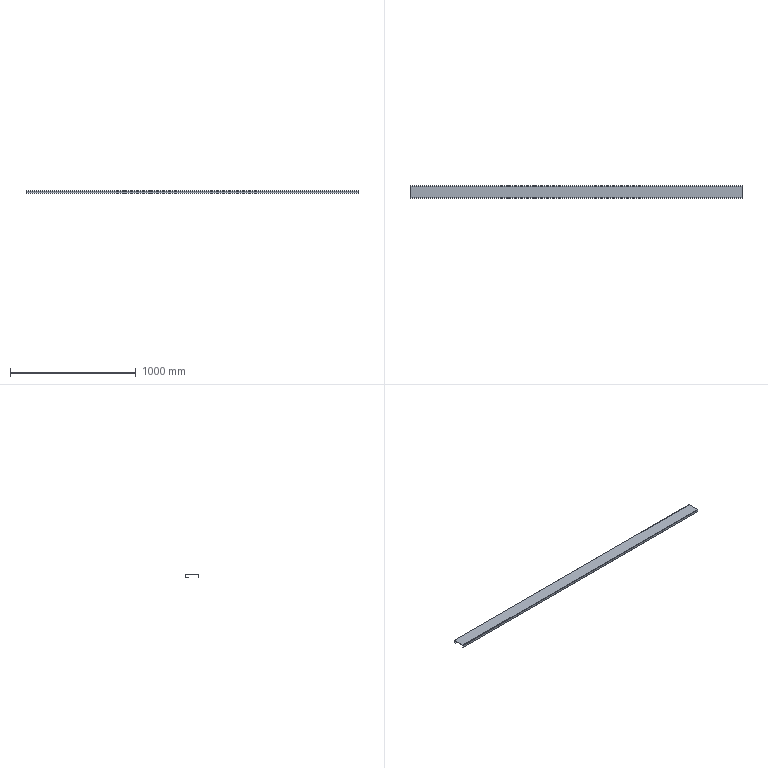Part | STEP file | E3-中转釜护栏2踢脚Plate | 1 solid | 18 faces | box 2640 x 100 x 20 mm | volume 606857 mm3 | plane 12 | cylinder 6 | commonest cylinder face diameters 2 x3 5 x3
STEP:
#1=CARTESIAN_POINT('',(0.,0.,0.));
#2=DIRECTION('',(0.,0.,1.));
#3=DIRECTION('',(1.,0.,0.));
#4=AXIS2_PLACEMENT_3D('',#1,#2,#3);
#5=CARTESIAN_POINT('',(-1320.,1.5,-2.5));
#6=VERTEX_POINT('',#5);
#7=CARTESIAN_POINT('',(-1320.,1.5,-20.));
#8=VERTEX_POINT('',#7);
#9=CARTESIAN_POINT('',(-1320.,1.5,-2.5));
#10=DIRECTION('',(0.,0.,-1.));
#11=VECTOR('',#10,1.);
#12=LINE('',#9,#11);
#13=CARTESIAN_POINT('',(1320.,1.5,-2.5));
#14=DIRECTION('',(0.,-1.,0.));
#15=DIRECTION('',(0.,0.,1.));
#16=AXIS2_PLACEMENT_3D('',#13,#14,#15);
#17=PLANE('',#16);
#18=CARTESIAN_POINT('',(0.,2640.));
#19=DIRECTION('',(-1.,0.));
#20=VECTOR('',#19,1.);
#21=LINE('',#18,#20);
#22=(GEOMETRIC_REPRESENTATION_CONTEXT(2)PARAMETRIC_REPRESENTATION_CONTEXT()REPRESENTATION_CONTEXT('',''));
#23=DEFINITIONAL_REPRESENTATION('',(#21),#22);
#24=PCURVE('',#17,#23);
#25=CARTESIAN_POINT('',(-1320.,2.5,-2.5));
#26=DIRECTION('',(-1.,0.,0.));
#27=DIRECTION('',(0.,0.,-1.));
#28=AXIS2_PLACEMENT_3D('',#25,#26,#27);
#29=PLANE('',#28);
#30=CARTESIAN_POINT('',(0.,1.));
#31=DIRECTION('',(1.,0.));
#32=VECTOR('',#31,1.);
#33=LINE('',#30,#32);
#34=(GEOMETRIC_REPRESENTATION_CONTEXT(2)PARAMETRIC_REPRESENTATION_CONTEXT()REPRESENTATION_CONTEXT('',''));
#35=DEFINITIONAL_REPRESENTATION('',(#33),#34);
#36=PCURVE('',#29,#35);
#37=SURFACE_CURVE('',#12,(#24,#36),.PCURVE_S1.);
#38=EDGE_CURVE('',#6,#8,#37,.T.);
#39=ORIENTED_EDGE('',*,*,#38,.F.);
#40=CARTESIAN_POINT('',(1320.,1.5,-2.5));
#41=VERTEX_POINT('',#40);
#42=CARTESIAN_POINT('',(1320.,1.5,-2.5));
#43=DIRECTION('',(-1.,0.,0.));
#44=VECTOR('',#43,1.);
#45=LINE('',#42,#44);
#46=CARTESIAN_POINT('',(0.,0.));
#47=DIRECTION('',(0.,1.));
#48=VECTOR('',#47,1.);
#49=LINE('',#46,#48);
#50=(GEOMETRIC_REPRESENTATION_CONTEXT(2)PARAMETRIC_REPRESENTATION_CONTEXT()REPRESENTATION_CONTEXT('',''));
#51=DEFINITIONAL_REPRESENTATION('',(#49),#50);
#52=PCURVE('',#17,#51);
#53=CARTESIAN_POINT('',(1320.,2.5,-2.5));
#54=DIRECTION('',(-1.,0.,0.));
#55=DIRECTION('',(0.,0.,-1.));
#56=AXIS2_PLACEMENT_3D('',#53,#54,#55);
#57=CYLINDRICAL_SURFACE('',#56,1.);
#58=CARTESIAN_POINT('',(1.571,0.));
#59=DIRECTION('',(0.,1.));
#60=VECTOR('',#59,1.);
#61=LINE('',#58,#60);
#62=(GEOMETRIC_REPRESENTATION_CONTEXT(2)PARAMETRIC_REPRESENTATION_CONTEXT()REPRESENTATION_CONTEXT('',''));
#63=DEFINITIONAL_REPRESENTATION('',(#61),#62);
#64=PCURVE('',#57,#63);
#65=SURFACE_CURVE('',#45,(#52,#64),.PCURVE_S1.);
#66=EDGE_CURVE('',#41,#6,#65,.T.);
#67=ORIENTED_EDGE('',*,*,#66,.F.);
#68=CARTESIAN_POINT('',(1320.,1.5,-20.));
#69=VERTEX_POINT('',#68);
#70=CARTESIAN_POINT('',(1320.,1.5,-2.5));
#71=DIRECTION('',(0.,0.,-1.));
#72=VECTOR('',#71,1.);
#73=LINE('',#70,#72);
#74=CARTESIAN_POINT('',(0.,0.));
#75=DIRECTION('',(-1.,0.));
#76=VECTOR('',#75,1.);
#77=LINE('',#74,#76);
#78=(GEOMETRIC_REPRESENTATION_CONTEXT(2)PARAMETRIC_REPRESENTATION_CONTEXT()REPRESENTATION_CONTEXT('',''));
#79=DEFINITIONAL_REPRESENTATION('',(#77),#78);
#80=PCURVE('',#17,#79);
#81=CARTESIAN_POINT('',(1320.,2.5,-2.5));
#82=DIRECTION('',(-1.,0.,0.));
#83=DIRECTION('',(0.,0.,-1.));
#84=AXIS2_PLACEMENT_3D('',#81,#82,#83);
#85=PLANE('',#84);
#86=CARTESIAN_POINT('',(0.,1.));
#87=DIRECTION('',(1.,0.));
#88=VECTOR('',#87,1.);
#89=LINE('',#86,#88);
#90=(GEOMETRIC_REPRESENTATION_CONTEXT(2)PARAMETRIC_REPRESENTATION_CONTEXT()REPRESENTATION_CONTEXT('',''));
#91=DEFINITIONAL_REPRESENTATION('',(#89),#90);
#92=PCURVE('',#85,#91);
#93=SURFACE_CURVE('',#73,(#80,#92),.PCURVE_S1.);
#94=EDGE_CURVE('',#41,#69,#93,.T.);
#95=ORIENTED_EDGE('',*,*,#94,.T.);
#96=CARTESIAN_POINT('',(1320.,1.5,-20.));
#97=DIRECTION('',(-1.,0.,0.));
#98=VECTOR('',#97,1.);
#99=LINE('',#96,#98);
#100=CARTESIAN_POINT('',(-17.5,0.));
#101=DIRECTION('',(0.,1.));
#102=VECTOR('',#101,1.);
#103=LINE('',#100,#102);
#104=(GEOMETRIC_REPRESENTATION_CONTEXT(2)PARAMETRIC_REPRESENTATION_CONTEXT()REPRESENTATION_CONTEXT('',''));
#105=DEFINITIONAL_REPRESENTATION('',(#103),#104);
#106=PCURVE('',#17,#105);
#107=CARTESIAN_POINT('',(1320.,0.,-20.));
#108=DIRECTION('',(0.,0.,-1.));
#109=DIRECTION('',(1.,0.,0.));
#110=AXIS2_PLACEMENT_3D('',#107,#108,#109);
#111=PLANE('',#110);
#112=CARTESIAN_POINT('',(0.,-1.5));
#113=DIRECTION('',(-1.,0.));
#114=VECTOR('',#113,1.);
#115=LINE('',#112,#114);
#116=(GEOMETRIC_REPRESENTATION_CONTEXT(2)PARAMETRIC_REPRESENTATION_CONTEXT()REPRESENTATION_CONTEXT('',''));
#117=DEFINITIONAL_REPRESENTATION('',(#115),#116);
#118=PCURVE('',#111,#117);
#119=SURFACE_CURVE('',#99,(#106,#118),.PCURVE_S1.);
#120=EDGE_CURVE('',#69,#8,#119,.T.);
#121=ORIENTED_EDGE('',*,*,#120,.T.);
#122=EDGE_LOOP('',(#39,#67,#95,#121));
#123=FACE_BOUND('',#122,.T.);
#124=ADVANCED_FACE('',(#123),#17,.F.);
#125=CARTESIAN_POINT('',(-1320.,0.,-20.));
#126=VERTEX_POINT('',#125);
#127=CARTESIAN_POINT('',(-1320.,0.,-20.));
#128=DIRECTION('',(0.,1.,0.));
#129=VECTOR('',#128,1.);
#130=LINE('',#127,#129);
#131=CARTESIAN_POINT('',(-2640.,0.));
#132=DIRECTION('',(0.,-1.));
#133=VECTOR('',#132,1.);
#134=LINE('',#131,#133);
#135=(GEOMETRIC_REPRESENTATION_CONTEXT(2)PARAMETRIC_REPRESENTATION_CONTEXT()REPRESENTATION_CONTEXT('',''));
#136=DEFINITIONAL_REPRESENTATION('',(#134),#135);
#137=PCURVE('',#111,#136);
#138=CARTESIAN_POINT('',(17.5,2.5));
#139=DIRECTION('',(0.,-1.));
#140=VECTOR('',#139,1.);
#141=LINE('',#138,#140);
#142=(GEOMETRIC_REPRESENTATION_CONTEXT(2)PARAMETRIC_REPRESENTATION_CONTEXT()REPRESENTATION_CONTEXT('',''));
#143=DEFINITIONAL_REPRESENTATION('',(#141),#142);
#144=PCURVE('',#29,#143);
#145=SURFACE_CURVE('',#130,(#137,#144),.PCURVE_S1.);
#146=EDGE_CURVE('',#126,#8,#145,.T.);
#147=ORIENTED_EDGE('',*,*,#146,.T.);
#148=ORIENTED_EDGE('',*,*,#120,.F.);
#149=CARTESIAN_POINT('',(1320.,0.,-20.));
#150=VERTEX_POINT('',#149);
#151=CARTESIAN_POINT('',(1320.,0.,-20.));
#152=DIRECTION('',(0.,1.,0.));
#153=VECTOR('',#152,1.);
#154=LINE('',#151,#153);
#155=CARTESIAN_POINT('',(0.,0.));
#156=DIRECTION('',(0.,-1.));
#157=VECTOR('',#156,1.);
#158=LINE('',#155,#157);
#159=(GEOMETRIC_REPRESENTATION_CONTEXT(2)PARAMETRIC_REPRESENTATION_CONTEXT()REPRESENTATION_CONTEXT('',''));
#160=DEFINITIONAL_REPRESENTATION('',(#158),#159);
#161=PCURVE('',#111,#160);
#162=CARTESIAN_POINT('',(17.5,2.5));
#163=DIRECTION('',(0.,-1.));
#164=VECTOR('',#163,1.);
#165=LINE('',#162,#164);
#166=(GEOMETRIC_REPRESENTATION_CONTEXT(2)PARAMETRIC_REPRESENTATION_CONTEXT()REPRESENTATION_CONTEXT('',''));
#167=DEFINITIONAL_REPRESENTATION('',(#165),#166);
#168=PCURVE('',#85,#167);
#169=SURFACE_CURVE('',#154,(#161,#168),.PCURVE_S1.);
#170=EDGE_CURVE('',#150,#69,#169,.T.);
#171=ORIENTED_EDGE('',*,*,#170,.F.);
#172=CARTESIAN_POINT('',(1320.,0.,-20.));
#173=DIRECTION('',(-1.,0.,0.));
#174=VECTOR('',#173,1.);
#175=LINE('',#172,#174);
#176=CARTESIAN_POINT('',(0.,0.));
#177=DIRECTION('',(-1.,0.));
#178=VECTOR('',#177,1.);
#179=LINE('',#176,#178);
#180=(GEOMETRIC_REPRESENTATION_CONTEXT(2)PARAMETRIC_REPRESENTATION_CONTEXT()REPRESENTATION_CONTEXT('',''));
#181=DEFINITIONAL_REPRESENTATION('',(#179),#180);
#182=PCURVE('',#111,#181);
#183=CARTESIAN_POINT('',(1320.,0.,-2.5));
#184=DIRECTION('',(0.,-1.,0.));
#185=DIRECTION('',(0.,0.,1.));
#186=AXIS2_PLACEMENT_3D('',#183,#184,#185);
#187=PLANE('',#186);
#188=CARTESIAN_POINT('',(-17.5,0.));
#189=DIRECTION('',(0.,1.));
#190=VECTOR('',#189,1.);
#191=LINE('',#188,#190);
#192=(GEOMETRIC_REPRESENTATION_CONTEXT(2)PARAMETRIC_REPRESENTATION_CONTEXT()REPRESENTATION_CONTEXT('',''));
#193=DEFINITIONAL_REPRESENTATION('',(#191),#192);
#194=PCURVE('',#187,#193);
#195=SURFACE_CURVE('',#175,(#182,#194),.PCURVE_S1.);
#196=EDGE_CURVE('',#150,#126,#195,.T.);
#197=ORIENTED_EDGE('',*,*,#196,.T.);
#198=EDGE_LOOP('',(#147,#148,#171,#197));
#199=FACE_BOUND('',#198,.T.);
#200=ADVANCED_FACE('',(#199),#111,.T.);
#201=CARTESIAN_POINT('',(-1320.,0.,-2.5));
#202=VERTEX_POINT('',#201);
#203=CARTESIAN_POINT('',(-1320.,0.,-2.5));
#204=DIRECTION('',(0.,0.,-1.));
#205=VECTOR('',#204,1.);
#206=LINE('',#203,#205);
#207=CARTESIAN_POINT('',(0.,2640.));
#208=DIRECTION('',(-1.,0.));
#209=VECTOR('',#208,1.);
#210=LINE('',#207,#209);
#211=(GEOMETRIC_REPRESENTATION_CONTEXT(2)PARAMETRIC_REPRESENTATION_CONTEXT()REPRESENTATION_CONTEXT('',''));
#212=DEFINITIONAL_REPRESENTATION('',(#210),#211);
#213=PCURVE('',#187,#212);
#214=CARTESIAN_POINT('',(0.,2.5));
#215=DIRECTION('',(1.,0.));
#216=VECTOR('',#215,1.);
#217=LINE('',#214,#216);
#218=(GEOMETRIC_REPRESENTATION_CONTEXT(2)PARAMETRIC_REPRESENTATION_CONTEXT()REPRESENTATION_CONTEXT('',''));
#219=DEFINITIONAL_REPRESENTATION('',(#217),#218);
#220=PCURVE('',#29,#219);
#221=SURFACE_CURVE('',#206,(#213,#220),.PCURVE_S1.);
#222=EDGE_CURVE('',#202,#126,#221,.T.);
#223=ORIENTED_EDGE('',*,*,#222,.T.);
#224=ORIENTED_EDGE('',*,*,#196,.F.);
#225=CARTESIAN_POINT('',(1320.,0.,-2.5));
#226=VERTEX_POINT('',#225);
#227=CARTESIAN_POINT('',(1320.,0.,-2.5));
#228=DIRECTION('',(0.,0.,-1.));
#229=VECTOR('',#228,1.);
#230=LINE('',#227,#229);
#231=CARTESIAN_POINT('',(0.,0.));
#232=DIRECTION('',(-1.,0.));
#233=VECTOR('',#232,1.);
#234=LINE('',#231,#233);
#235=(GEOMETRIC_REPRESENTATION_CONTEXT(2)PARAMETRIC_REPRESENTATION_CONTEXT()REPRESENTATION_CONTEXT('',''));
#236=DEFINITIONAL_REPRESENTATION('',(#234),#235);
#237=PCURVE('',#187,#236);
#238=CARTESIAN_POINT('',(0.,2.5));
#239=DIRECTION('',(1.,0.));
#240=VECTOR('',#239,1.);
#241=LINE('',#238,#240);
#242=(GEOMETRIC_REPRESENTATION_CONTEXT(2)PARAMETRIC_REPRESENTATION_CONTEXT()REPRESENTATION_CONTEXT('',''));
#243=DEFINITIONAL_REPRESENTATION('',(#241),#242);
#244=PCURVE('',#85,#243);
#245=SURFACE_CURVE('',#230,(#237,#244),.PCURVE_S1.);
#246=EDGE_CURVE('',#226,#150,#245,.T.);
#247=ORIENTED_EDGE('',*,*,#246,.F.);
#248=CARTESIAN_POINT('',(1320.,0.,-2.5));
#249=DIRECTION('',(-1.,0.,0.));
#250=VECTOR('',#249,1.);
#251=LINE('',#248,#250);
#252=CARTESIAN_POINT('',(0.,0.));
#253=DIRECTION('',(0.,1.));
#254=VECTOR('',#253,1.);
#255=LINE('',#252,#254);
#256=(GEOMETRIC_REPRESENTATION_CONTEXT(2)PARAMETRIC_REPRESENTATION_CONTEXT()REPRESENTATION_CONTEXT('',''));
#257=DEFINITIONAL_REPRESENTATION('',(#255),#256);
#258=PCURVE('',#187,#257);
#259=CARTESIAN_POINT('',(1320.,2.5,-2.5));
#260=DIRECTION('',(-1.,0.,0.));
#261=DIRECTION('',(0.,0.,-1.));
#262=AXIS2_PLACEMENT_3D('',#259,#260,#261);
#263=CYLINDRICAL_SURFACE('',#262,2.5);
#264=CARTESIAN_POINT('',(1.571,0.));
#265=DIRECTION('',(0.,1.));
#266=VECTOR('',#265,1.);
#267=LINE('',#264,#266);
#268=(GEOMETRIC_REPRESENTATION_CONTEXT(2)PARAMETRIC_REPRESENTATION_CONTEXT()REPRESENTATION_CONTEXT('',''));
#269=DEFINITIONAL_REPRESENTATION('',(#267),#268);
#270=PCURVE('',#263,#269);
#271=SURFACE_CURVE('',#251,(#258,#270),.PCURVE_S1.);
#272=EDGE_CURVE('',#226,#202,#271,.T.);
#273=ORIENTED_EDGE('',*,*,#272,.T.);
#274=EDGE_LOOP('',(#223,#224,#247,#273));
#275=FACE_BOUND('',#274,.T.);
#276=ADVANCED_FACE('',(#275),#187,.T.);
#277=CARTESIAN_POINT('',(-1320.,2.5,0.));
#278=VERTEX_POINT('',#277);
#279=CARTESIAN_POINT('',(-1320.,2.5,-2.5));
#280=DIRECTION('',(1.,0.,0.));
#281=DIRECTION('',(0.,0.,-1.));
#282=AXIS2_PLACEMENT_3D('',#279,#280,#281);
#283=CIRCLE('',#282,2.5);
#284=CARTESIAN_POINT('',(6.283,2640.));
#285=DIRECTION('',(-1.,0.));
#286=VECTOR('',#285,1.);
#287=LINE('',#284,#286);
#288=(GEOMETRIC_REPRESENTATION_CONTEXT(2)PARAMETRIC_REPRESENTATION_CONTEXT()REPRESENTATION_CONTEXT('',''));
#289=DEFINITIONAL_REPRESENTATION('',(#287),#288);
#290=PCURVE('',#263,#289);
#291=CARTESIAN_POINT('',(2.5,0.));
#292=CARTESIAN_POINT('',(2.5,-4.33));
#293=CARTESIAN_POINT('',(-1.25,-2.165));
#294=CARTESIAN_POINT('',(-5.,0.));
#295=CARTESIAN_POINT('',(-1.25,2.165));
#296=CARTESIAN_POINT('',(2.5,4.33));
#297=CARTESIAN_POINT('',(2.5,0.));
#298=(BOUNDED_CURVE()B_SPLINE_CURVE(2,(#291,#292,#293,#294,#295,#296,#297),.UNSPECIFIED.,.T.,.F.)B_SPLINE_CURVE_WITH_KNOTS((1,2,2,2,2,1),(-2.094,0.,2.094,4.189,6.283,8.378),.UNSPECIFIED.)CURVE()GEOMETRIC_REPRESENTATION_ITEM()RATIONAL_B_SPLINE_CURVE((1.,0.5,1.,0.5,1.,0.5,1.))REPRESENTATION_ITEM(''));
#299=(GEOMETRIC_REPRESENTATION_CONTEXT(2)PARAMETRIC_REPRESENTATION_CONTEXT()REPRESENTATION_CONTEXT('',''));
#300=DEFINITIONAL_REPRESENTATION('',(#298),#299);
#301=PCURVE('',#29,#300);
#302=SURFACE_CURVE('',#283,(#290,#301),.PCURVE_S1.);
#303=EDGE_CURVE('',#278,#202,#302,.T.);
#304=ORIENTED_EDGE('',*,*,#303,.T.);
#305=ORIENTED_EDGE('',*,*,#272,.F.);
#306=CARTESIAN_POINT('',(1320.,2.5,0.));
#307=VERTEX_POINT('',#306);
#308=CARTESIAN_POINT('',(1320.,2.5,-2.5));
#309=DIRECTION('',(1.,0.,0.));
#310=DIRECTION('',(0.,0.,-1.));
#311=AXIS2_PLACEMENT_3D('',#308,#309,#310);
#312=CIRCLE('',#311,2.5);
#313=CARTESIAN_POINT('',(6.283,0.));
#314=DIRECTION('',(-1.,0.));
#315=VECTOR('',#314,1.);
#316=LINE('',#313,#315);
#317=(GEOMETRIC_REPRESENTATION_CONTEXT(2)PARAMETRIC_REPRESENTATION_CONTEXT()REPRESENTATION_CONTEXT('',''));
#318=DEFINITIONAL_REPRESENTATION('',(#316),#317);
#319=PCURVE('',#263,#318);
#320=CARTESIAN_POINT('',(2.5,0.));
#321=CARTESIAN_POINT('',(2.5,-4.33));
#322=CARTESIAN_POINT('',(-1.25,-2.165));
#323=CARTESIAN_POINT('',(-5.,0.));
#324=CARTESIAN_POINT('',(-1.25,2.165));
#325=CARTESIAN_POINT('',(2.5,4.33));
#326=CARTESIAN_POINT('',(2.5,0.));
#327=(BOUNDED_CURVE()B_SPLINE_CURVE(2,(#320,#321,#322,#323,#324,#325,#326),.UNSPECIFIED.,.T.,.F.)B_SPLINE_CURVE_WITH_KNOTS((1,2,2,2,2,1),(-2.094,0.,2.094,4.189,6.283,8.378),.UNSPECIFIED.)CURVE()GEOMETRIC_REPRESENTATION_ITEM()RATIONAL_B_SPLINE_CURVE((1.,0.5,1.,0.5,1.,0.5,1.))REPRESENTATION_ITEM(''));
#328=(GEOMETRIC_REPRESENTATION_CONTEXT(2)PARAMETRIC_REPRESENTATION_CONTEXT()REPRESENTATION_CONTEXT('',''));
#329=DEFINITIONAL_REPRESENTATION('',(#327),#328);
#330=PCURVE('',#85,#329);
#331=SURFACE_CURVE('',#312,(#319,#330),.PCURVE_S1.);
#332=EDGE_CURVE('',#307,#226,#331,.T.);
#333=ORIENTED_EDGE('',*,*,#332,.F.);
#334=CARTESIAN_POINT('',(1320.,2.5,0.));
#335=DIRECTION('',(-1.,0.,0.));
#336=VECTOR('',#335,1.);
#337=LINE('',#334,#336);
#338=CARTESIAN_POINT('',(3.142,0.));
#339=DIRECTION('',(0.,1.));
#340=VECTOR('',#339,1.);
#341=LINE('',#338,#340);
#342=(GEOMETRIC_REPRESENTATION_CONTEXT(2)PARAMETRIC_REPRESENTATION_CONTEXT()REPRESENTATION_CONTEXT('',''));
#343=DEFINITIONAL_REPRESENTATION('',(#341),#342);
#344=PCURVE('',#263,#343);
#345=CARTESIAN_POINT('',(1320.,2.5,0.));
#346=DIRECTION('',(0.,0.,1.));
#347=DIRECTION('',(-1.,0.,0.));
#348=AXIS2_PLACEMENT_3D('',#345,#346,#347);
#349=PLANE('',#348);
#350=CARTESIAN_POINT('',(0.,0.));
#351=DIRECTION('',(1.,0.));
#352=VECTOR('',#351,1.);
#353=LINE('',#350,#352);
#354=(GEOMETRIC_REPRESENTATION_CONTEXT(2)PARAMETRIC_REPRESENTATION_CONTEXT()REPRESENTATION_CONTEXT('',''));
#355=DEFINITIONAL_REPRESENTATION('',(#353),#354);
#356=PCURVE('',#349,#355);
#357=SURFACE_CURVE('',#337,(#344,#356),.PCURVE_S1.);
#358=EDGE_CURVE('',#307,#278,#357,.T.);
#359=ORIENTED_EDGE('',*,*,#358,.T.);
#360=EDGE_LOOP('',(#304,#305,#333,#359));
#361=FACE_BOUND('',#360,.T.);
#362=ADVANCED_FACE('',(#361),#263,.T.);
#363=CARTESIAN_POINT('',(-1320.,97.5,0.));
#364=VERTEX_POINT('',#363);
#365=CARTESIAN_POINT('',(-1320.,2.5,0.));
#366=DIRECTION('',(0.,-1.,0.));
#367=VECTOR('',#366,1.);
#368=LINE('',#365,#367);
#369=CARTESIAN_POINT('',(2640.,0.));
#370=DIRECTION('',(0.,1.));
#371=VECTOR('',#370,1.);
#372=LINE('',#369,#371);
#373=(GEOMETRIC_REPRESENTATION_CONTEXT(2)PARAMETRIC_REPRESENTATION_CONTEXT()REPRESENTATION_CONTEXT('',''));
#374=DEFINITIONAL_REPRESENTATION('',(#372),#373);
#375=PCURVE('',#349,#374);
#376=CARTESIAN_POINT('',(-2.5,0.));
#377=DIRECTION('',(0.,1.));
#378=VECTOR('',#377,1.);
#379=LINE('',#376,#378);
#380=(GEOMETRIC_REPRESENTATION_CONTEXT(2)PARAMETRIC_REPRESENTATION_CONTEXT()REPRESENTATION_CONTEXT('',''));
#381=DEFINITIONAL_REPRESENTATION('',(#379),#380);
#382=PCURVE('',#29,#381);
#383=SURFACE_CURVE('',#368,(#375,#382),.PCURVE_S1.);
#384=EDGE_CURVE('',#364,#278,#383,.T.);
#385=ORIENTED_EDGE('',*,*,#384,.T.);
#386=ORIENTED_EDGE('',*,*,#358,.F.);
#387=CARTESIAN_POINT('',(1320.,97.5,0.));
#388=VERTEX_POINT('',#387);
#389=CARTESIAN_POINT('',(1320.,2.5,0.));
#390=DIRECTION('',(0.,-1.,0.));
#391=VECTOR('',#390,1.);
#392=LINE('',#389,#391);
#393=CARTESIAN_POINT('',(0.,0.));
#394=DIRECTION('',(0.,1.));
#395=VECTOR('',#394,1.);
#396=LINE('',#393,#395);
#397=(GEOMETRIC_REPRESENTATION_CONTEXT(2)PARAMETRIC_REPRESENTATION_CONTEXT()REPRESENTATION_CONTEXT('',''));
#398=DEFINITIONAL_REPRESENTATION('',(#396),#397);
#399=PCURVE('',#349,#398);
#400=CARTESIAN_POINT('',(-2.5,0.));
#401=DIRECTION('',(0.,1.));
#402=VECTOR('',#401,1.);
#403=LINE('',#400,#402);
#404=(GEOMETRIC_REPRESENTATION_CONTEXT(2)PARAMETRIC_REPRESENTATION_CONTEXT()REPRESENTATION_CONTEXT('',''));
#405=DEFINITIONAL_REPRESENTATION('',(#403),#404);
#406=PCURVE('',#85,#405);
#407=SURFACE_CURVE('',#392,(#399,#406),.PCURVE_S1.);
#408=EDGE_CURVE('',#388,#307,#407,.T.);
#409=ORIENTED_EDGE('',*,*,#408,.F.);
#410=CARTESIAN_POINT('',(1320.,97.5,0.));
#411=DIRECTION('',(-1.,0.,0.));
#412=VECTOR('',#411,1.);
#413=LINE('',#410,#412);
#414=CARTESIAN_POINT('',(0.,-95.));
#415=DIRECTION('',(1.,0.));
#416=VECTOR('',#415,1.);
#417=LINE('',#414,#416);
#418=(GEOMETRIC_REPRESENTATION_CONTEXT(2)PARAMETRIC_REPRESENTATION_CONTEXT()REPRESENTATION_CONTEXT('',''));
#419=DEFINITIONAL_REPRESENTATION('',(#417),#418);
#420=PCURVE('',#349,#419);
#421=CARTESIAN_POINT('',(1320.,97.5,-2.5));
#422=DIRECTION('',(-1.,0.,0.));
#423=DIRECTION('',(0.,0.,-1.));
#424=AXIS2_PLACEMENT_3D('',#421,#422,#423);
#425=CYLINDRICAL_SURFACE('',#424,2.5);
#426=CARTESIAN_POINT('',(3.142,0.));
#427=DIRECTION('',(0.,1.));
#428=VECTOR('',#427,1.);
#429=LINE('',#426,#428);
#430=(GEOMETRIC_REPRESENTATION_CONTEXT(2)PARAMETRIC_REPRESENTATION_CONTEXT()REPRESENTATION_CONTEXT('',''));
#431=DEFINITIONAL_REPRESENTATION('',(#429),#430);
#432=PCURVE('',#425,#431);
#433=SURFACE_CURVE('',#413,(#420,#432),.PCURVE_S1.);
#434=EDGE_CURVE('',#388,#364,#433,.T.);
#435=ORIENTED_EDGE('',*,*,#434,.T.);
#436=EDGE_LOOP('',(#385,#386,#409,#435));
#437=FACE_BOUND('',#436,.T.);
#438=ADVANCED_FACE('',(#437),#349,.T.);
#439=CARTESIAN_POINT('',(-1320.,100.,-2.5));
#440=VERTEX_POINT('',#439);
#441=CARTESIAN_POINT('',(-1320.,97.5,-2.5));
#442=DIRECTION('',(1.,0.,0.));
#443=DIRECTION('',(0.,0.,1.));
#444=AXIS2_PLACEMENT_3D('',#441,#442,#443);
#445=CIRCLE('',#444,2.5);
#446=CARTESIAN_POINT('',(9.425,2640.));
#447=DIRECTION('',(-1.,0.));
#448=VECTOR('',#447,1.);
#449=LINE('',#446,#448);
#450=(GEOMETRIC_REPRESENTATION_CONTEXT(2)PARAMETRIC_REPRESENTATION_CONTEXT()REPRESENTATION_CONTEXT('',''));
#451=DEFINITIONAL_REPRESENTATION('',(#449),#450);
#452=PCURVE('',#425,#451);
#453=CARTESIAN_POINT('',(-2.5,-95.));
#454=CARTESIAN_POINT('',(-2.5,-90.67));
#455=CARTESIAN_POINT('',(1.25,-92.835));
#456=CARTESIAN_POINT('',(5.,-95.));
#457=CARTESIAN_POINT('',(1.25,-97.165));
#458=CARTESIAN_POINT('',(-2.5,-99.33));
#459=CARTESIAN_POINT('',(-2.5,-95.));
#460=(BOUNDED_CURVE()B_SPLINE_CURVE(2,(#453,#454,#455,#456,#457,#458,#459),.UNSPECIFIED.,.T.,.F.)B_SPLINE_CURVE_WITH_KNOTS((1,2,2,2,2,1),(-2.094,0.,2.094,4.189,6.283,8.378),.UNSPECIFIED.)CURVE()GEOMETRIC_REPRESENTATION_ITEM()RATIONAL_B_SPLINE_CURVE((1.,0.5,1.,0.5,1.,0.5,1.))REPRESENTATION_ITEM(''));
#461=(GEOMETRIC_REPRESENTATION_CONTEXT(2)PARAMETRIC_REPRESENTATION_CONTEXT()REPRESENTATION_CONTEXT('',''));
#462=DEFINITIONAL_REPRESENTATION('',(#460),#461);
#463=PCURVE('',#29,#462);
#464=SURFACE_CURVE('',#445,(#452,#463),.PCURVE_S1.);
#465=EDGE_CURVE('',#440,#364,#464,.T.);
#466=ORIENTED_EDGE('',*,*,#465,.T.);
#467=ORIENTED_EDGE('',*,*,#434,.F.);
#468=CARTESIAN_POINT('',(1320.,100.,-2.5));
#469=VERTEX_POINT('',#468);
#470=CARTESIAN_POINT('',(1320.,97.5,-2.5));
#471=DIRECTION('',(1.,0.,0.));
#472=DIRECTION('',(0.,0.,1.));
#473=AXIS2_PLACEMENT_3D('',#470,#471,#472);
#474=CIRCLE('',#473,2.5);
#475=CARTESIAN_POINT('',(9.425,0.));
#476=DIRECTION('',(-1.,0.));
#477=VECTOR('',#476,1.);
#478=LINE('',#475,#477);
#479=(GEOMETRIC_REPRESENTATION_CONTEXT(2)PARAMETRIC_REPRESENTATION_CONTEXT()REPRESENTATION_CONTEXT('',''));
#480=DEFINITIONAL_REPRESENTATION('',(#478),#479);
#481=PCURVE('',#425,#480);
#482=CARTESIAN_POINT('',(-2.5,-95.));
#483=CARTESIAN_POINT('',(-2.5,-90.67));
#484=CARTESIAN_POINT('',(1.25,-92.835));
#485=CARTESIAN_POINT('',(5.,-95.));
#486=CARTESIAN_POINT('',(1.25,-97.165));
#487=CARTESIAN_POINT('',(-2.5,-99.33));
#488=CARTESIAN_POINT('',(-2.5,-95.));
#489=(BOUNDED_CURVE()B_SPLINE_CURVE(2,(#482,#483,#484,#485,#486,#487,#488),.UNSPECIFIED.,.T.,.F.)B_SPLINE_CURVE_WITH_KNOTS((1,2,2,2,2,1),(-2.094,0.,2.094,4.189,6.283,8.378),.UNSPECIFIED.)CURVE()GEOMETRIC_REPRESENTATION_ITEM()RATIONAL_B_SPLINE_CURVE((1.,0.5,1.,0.5,1.,0.5,1.))REPRESENTATION_ITEM(''));
#490=(GEOMETRIC_REPRESENTATION_CONTEXT(2)PARAMETRIC_REPRESENTATION_CONTEXT()REPRESENTATION_CONTEXT('',''));
#491=DEFINITIONAL_REPRESENTATION('',(#489),#490);
#492=PCURVE('',#85,#491);
#493=SURFACE_CURVE('',#474,(#481,#492),.PCURVE_S1.);
#494=EDGE_CURVE('',#469,#388,#493,.T.);
#495=ORIENTED_EDGE('',*,*,#494,.F.);
#496=CARTESIAN_POINT('',(1320.,100.,-2.5));
#497=DIRECTION('',(-1.,0.,0.));
#498=VECTOR('',#497,1.);
#499=LINE('',#496,#498);
#500=CARTESIAN_POINT('',(4.712,0.));
#501=DIRECTION('',(0.,1.));
#502=VECTOR('',#501,1.);
#503=LINE('',#500,#502);
#504=(GEOMETRIC_REPRESENTATION_CONTEXT(2)PARAMETRIC_REPRESENTATION_CONTEXT()REPRESENTATION_CONTEXT('',''));
#505=DEFINITIONAL_REPRESENTATION('',(#503),#504);
#506=PCURVE('',#425,#505);
#507=CARTESIAN_POINT('',(1320.,100.,-2.5));
#508=DIRECTION('',(0.,1.,0.));
#509=DIRECTION('',(0.,0.,-1.));
#510=AXIS2_PLACEMENT_3D('',#507,#508,#509);
#511=PLANE('',#510);
#512=CARTESIAN_POINT('',(0.,0.));
#513=DIRECTION('',(0.,1.));
#514=VECTOR('',#513,1.);
#515=LINE('',#512,#514);
#516=(GEOMETRIC_REPRESENTATION_CONTEXT(2)PARAMETRIC_REPRESENTATION_CONTEXT()REPRESENTATION_CONTEXT('',''));
#517=DEFINITIONAL_REPRESENTATION('',(#515),#516);
#518=PCURVE('',#511,#517);
#519=SURFACE_CURVE('',#499,(#506,#518),.PCURVE_S1.);
#520=EDGE_CURVE('',#469,#440,#519,.T.);
#521=ORIENTED_EDGE('',*,*,#520,.T.);
#522=EDGE_LOOP('',(#466,#467,#495,#521));
#523=FACE_BOUND('',#522,.T.);
#524=ADVANCED_FACE('',(#523),#425,.T.);
#525=CARTESIAN_POINT('',(-1320.,100.,-17.5));
#526=VERTEX_POINT('',#525);
#527=CARTESIAN_POINT('',(-1320.,100.,-2.5));
#528=DIRECTION('',(0.,0.,1.));
#529=VECTOR('',#528,1.);
#530=LINE('',#527,#529);
#531=CARTESIAN_POINT('',(0.,2640.));
#532=DIRECTION('',(-1.,0.));
#533=VECTOR('',#532,1.);
#534=LINE('',#531,#533);
#535=(GEOMETRIC_REPRESENTATION_CONTEXT(2)PARAMETRIC_REPRESENTATION_CONTEXT()REPRESENTATION_CONTEXT('',''));
#536=DEFINITIONAL_REPRESENTATION('',(#534),#535);
#537=PCURVE('',#511,#536);
#538=CARTESIAN_POINT('',(0.,-97.5));
#539=DIRECTION('',(-1.,0.));
#540=VECTOR('',#539,1.);
#541=LINE('',#538,#540);
#542=(GEOMETRIC_REPRESENTATION_CONTEXT(2)PARAMETRIC_REPRESENTATION_CONTEXT()REPRESENTATION_CONTEXT('',''));
#543=DEFINITIONAL_REPRESENTATION('',(#541),#542);
#544=PCURVE('',#29,#543);
#545=SURFACE_CURVE('',#530,(#537,#544),.PCURVE_S1.);
#546=EDGE_CURVE('',#526,#440,#545,.T.);
#547=ORIENTED_EDGE('',*,*,#546,.T.);
#548=ORIENTED_EDGE('',*,*,#520,.F.);
#549=CARTESIAN_POINT('',(1320.,100.,-17.5));
#550=VERTEX_POINT('',#549);
#551=CARTESIAN_POINT('',(1320.,100.,-2.5));
#552=DIRECTION('',(0.,0.,1.));
#553=VECTOR('',#552,1.);
#554=LINE('',#551,#553);
#555=CARTESIAN_POINT('',(0.,0.));
#556=DIRECTION('',(-1.,0.));
#557=VECTOR('',#556,1.);
#558=LINE('',#555,#557);
#559=(GEOMETRIC_REPRESENTATION_CONTEXT(2)PARAMETRIC_REPRESENTATION_CONTEXT()REPRESENTATION_CONTEXT('',''));
#560=DEFINITIONAL_REPRESENTATION('',(#558),#559);
#561=PCURVE('',#511,#560);
#562=CARTESIAN_POINT('',(0.,-97.5));
#563=DIRECTION('',(-1.,0.));
#564=VECTOR('',#563,1.);
#565=LINE('',#562,#564);
#566=(GEOMETRIC_REPRESENTATION_CONTEXT(2)PARAMETRIC_REPRESENTATION_CONTEXT()REPRESENTATION_CONTEXT('',''));
#567=DEFINITIONAL_REPRESENTATION('',(#565),#566);
#568=PCURVE('',#85,#567);
#569=SURFACE_CURVE('',#554,(#561,#568),.PCURVE_S1.);
#570=EDGE_CURVE('',#550,#469,#569,.T.);
#571=ORIENTED_EDGE('',*,*,#570,.F.);
#572=CARTESIAN_POINT('',(1320.,100.,-17.5));
#573=DIRECTION('',(-1.,0.,0.));
#574=VECTOR('',#573,1.);
#575=LINE('',#572,#574);
#576=CARTESIAN_POINT('',(15.,0.));
#577=DIRECTION('',(0.,1.));
#578=VECTOR('',#577,1.);
#579=LINE('',#576,#578);
#580=(GEOMETRIC_REPRESENTATION_CONTEXT(2)PARAMETRIC_REPRESENTATION_CONTEXT()REPRESENTATION_CONTEXT('',''));
#581=DEFINITIONAL_REPRESENTATION('',(#579),#580);
#582=PCURVE('',#511,#581);
#583=CARTESIAN_POINT('',(1320.,97.5,-17.5));
#584=DIRECTION('',(-1.,0.,0.));
#585=DIRECTION('',(0.,0.,-1.));
#586=AXIS2_PLACEMENT_3D('',#583,#584,#585);
#587=CYLINDRICAL_SURFACE('',#586,2.5);
#588=CARTESIAN_POINT('',(4.712,0.));
#589=DIRECTION('',(0.,1.));
#590=VECTOR('',#589,1.);
#591=LINE('',#588,#590);
#592=(GEOMETRIC_REPRESENTATION_CONTEXT(2)PARAMETRIC_REPRESENTATION_CONTEXT()REPRESENTATION_CONTEXT('',''));
#593=DEFINITIONAL_REPRESENTATION('',(#591),#592);
#594=PCURVE('',#587,#593);
#595=SURFACE_CURVE('',#575,(#582,#594),.PCURVE_S1.);
#596=EDGE_CURVE('',#550,#526,#595,.T.);
#597=ORIENTED_EDGE('',*,*,#596,.T.);
#598=EDGE_LOOP('',(#547,#548,#571,#597));
#599=FACE_BOUND('',#598,.T.);
#600=ADVANCED_FACE('',(#599),#511,.T.);
#601=CARTESIAN_POINT('',(-1320.,97.5,-20.));
#602=VERTEX_POINT('',#601);
#603=CARTESIAN_POINT('',(-1320.,97.5,-17.5));
#604=DIRECTION('',(1.,0.,0.));
#605=DIRECTION('',(0.,0.,1.));
#606=AXIS2_PLACEMENT_3D('',#603,#604,#605);
#607=CIRCLE('',#606,2.5);
#608=CARTESIAN_POINT('',(9.425,2640.));
#609=DIRECTION('',(-1.,0.));
#610=VECTOR('',#609,1.);
#611=LINE('',#608,#610);
#612=(GEOMETRIC_REPRESENTATION_CONTEXT(2)PARAMETRIC_REPRESENTATION_CONTEXT()REPRESENTATION_CONTEXT('',''));
#613=DEFINITIONAL_REPRESENTATION('',(#611),#612);
#614=PCURVE('',#587,#613);
#615=CARTESIAN_POINT('',(12.5,-95.));
#616=CARTESIAN_POINT('',(12.5,-90.67));
#617=CARTESIAN_POINT('',(16.25,-92.835));
#618=CARTESIAN_POINT('',(20.,-95.));
#619=CARTESIAN_POINT('',(16.25,-97.165));
#620=CARTESIAN_POINT('',(12.5,-99.33));
#621=CARTESIAN_POINT('',(12.5,-95.));
#622=(BOUNDED_CURVE()B_SPLINE_CURVE(2,(#615,#616,#617,#618,#619,#620,#621),.UNSPECIFIED.,.T.,.F.)B_SPLINE_CURVE_WITH_KNOTS((1,2,2,2,2,1),(-2.094,0.,2.094,4.189,6.283,8.378),.UNSPECIFIED.)CURVE()GEOMETRIC_REPRESENTATION_ITEM()RATIONAL_B_SPLINE_CURVE((1.,0.5,1.,0.5,1.,0.5,1.))REPRESENTATION_ITEM(''));
#623=(GEOMETRIC_REPRESENTATION_CONTEXT(2)PARAMETRIC_REPRESENTATION_CONTEXT()REPRESENTATION_CONTEXT('',''));
#624=DEFINITIONAL_REPRESENTATION('',(#622),#623);
#625=PCURVE('',#29,#624);
#626=SURFACE_CURVE('',#607,(#614,#625),.PCURVE_S1.);
#627=EDGE_CURVE('',#602,#526,#626,.T.);
#628=ORIENTED_EDGE('',*,*,#627,.T.);
#629=ORIENTED_EDGE('',*,*,#596,.F.);
#630=CARTESIAN_POINT('',(1320.,97.5,-20.));
#631=VERTEX_POINT('',#630);
#632=CARTESIAN_POINT('',(1320.,97.5,-17.5));
#633=DIRECTION('',(1.,0.,0.));
#634=DIRECTION('',(0.,0.,1.));
#635=AXIS2_PLACEMENT_3D('',#632,#633,#634);
#636=CIRCLE('',#635,2.5);
#637=CARTESIAN_POINT('',(9.425,0.));
#638=DIRECTION('',(-1.,0.));
#639=VECTOR('',#638,1.);
#640=LINE('',#637,#639);
#641=(GEOMETRIC_REPRESENTATION_CONTEXT(2)PARAMETRIC_REPRESENTATION_CONTEXT()REPRESENTATION_CONTEXT('',''));
#642=DEFINITIONAL_REPRESENTATION('',(#640),#641);
#643=PCURVE('',#587,#642);
#644=CARTESIAN_POINT('',(12.5,-95.));
#645=CARTESIAN_POINT('',(12.5,-90.67));
#646=CARTESIAN_POINT('',(16.25,-92.835));
#647=CARTESIAN_POINT('',(20.,-95.));
#648=CARTESIAN_POINT('',(16.25,-97.165));
#649=CARTESIAN_POINT('',(12.5,-99.33));
#650=CARTESIAN_POINT('',(12.5,-95.));
#651=(BOUNDED_CURVE()B_SPLINE_CURVE(2,(#644,#645,#646,#647,#648,#649,#650),.UNSPECIFIED.,.T.,.F.)B_SPLINE_CURVE_WITH_KNOTS((1,2,2,2,2,1),(-2.094,0.,2.094,4.189,6.283,8.378),.UNSPECIFIED.)CURVE()GEOMETRIC_REPRESENTATION_ITEM()RATIONAL_B_SPLINE_CURVE((1.,0.5,1.,0.5,1.,0.5,1.))REPRESENTATION_ITEM(''));
#652=(GEOMETRIC_REPRESENTATION_CONTEXT(2)PARAMETRIC_REPRESENTATION_CONTEXT()REPRESENTATION_CONTEXT('',''));
#653=DEFINITIONAL_REPRESENTATION('',(#651),#652);
#654=PCURVE('',#85,#653);
#655=SURFACE_CURVE('',#636,(#643,#654),.PCURVE_S1.);
#656=EDGE_CURVE('',#631,#550,#655,.T.);
#657=ORIENTED_EDGE('',*,*,#656,.F.);
#658=CARTESIAN_POINT('',(1320.,97.5,-20.));
#659=DIRECTION('',(-1.,0.,0.));
#660=VECTOR('',#659,1.);
#661=LINE('',#658,#660);
#662=CARTESIAN_POINT('',(6.283,0.));
#663=DIRECTION('',(0.,1.));
#664=VECTOR('',#663,1.);
#665=LINE('',#662,#664);
#666=(GEOMETRIC_REPRESENTATION_CONTEXT(2)PARAMETRIC_REPRESENTATION_CONTEXT()REPRESENTATION_CONTEXT('',''));
#667=DEFINITIONAL_REPRESENTATION('',(#665),#666);
#668=PCURVE('',#587,#667);
#669=CARTESIAN_POINT('',(1320.,97.5,-20.));
#670=DIRECTION('',(0.,0.,-1.));
#671=DIRECTION('',(1.,0.,0.));
#672=AXIS2_PLACEMENT_3D('',#669,#670,#671);
#673=PLANE('',#672);
#674=CARTESIAN_POINT('',(0.,0.));
#675=DIRECTION('',(-1.,0.));
#676=VECTOR('',#675,1.);
#677=LINE('',#674,#676);
#678=(GEOMETRIC_REPRESENTATION_CONTEXT(2)PARAMETRIC_REPRESENTATION_CONTEXT()REPRESENTATION_CONTEXT('',''));
#679=DEFINITIONAL_REPRESENTATION('',(#677),#678);
#680=PCURVE('',#673,#679);
#681=SURFACE_CURVE('',#661,(#668,#680),.PCURVE_S1.);
#682=EDGE_CURVE('',#631,#602,#681,.T.);
#683=ORIENTED_EDGE('',*,*,#682,.T.);
#684=EDGE_LOOP('',(#628,#629,#657,#683));
#685=FACE_BOUND('',#684,.T.);
#686=ADVANCED_FACE('',(#685),#587,.T.);
#687=CARTESIAN_POINT('',(-1320.,80.,-20.));
#688=VERTEX_POINT('',#687);
#689=CARTESIAN_POINT('',(-1320.,97.5,-20.));
#690=DIRECTION('',(0.,1.,0.));
#691=VECTOR('',#690,1.);
#692=LINE('',#689,#691);
#693=CARTESIAN_POINT('',(-2640.,0.));
#694=DIRECTION('',(0.,-1.));
#695=VECTOR('',#694,1.);
#696=LINE('',#693,#695);
#697=(GEOMETRIC_REPRESENTATION_CONTEXT(2)PARAMETRIC_REPRESENTATION_CONTEXT()REPRESENTATION_CONTEXT('',''));
#698=DEFINITIONAL_REPRESENTATION('',(#696),#697);
#699=PCURVE('',#673,#698);
#700=CARTESIAN_POINT('',(17.5,-95.));
#701=DIRECTION('',(0.,-1.));
#702=VECTOR('',#701,1.);
#703=LINE('',#700,#702);
#704=(GEOMETRIC_REPRESENTATION_CONTEXT(2)PARAMETRIC_REPRESENTATION_CONTEXT()REPRESENTATION_CONTEXT('',''));
#705=DEFINITIONAL_REPRESENTATION('',(#703),#704);
#706=PCURVE('',#29,#705);
#707=SURFACE_CURVE('',#692,(#699,#706),.PCURVE_S1.);
#708=EDGE_CURVE('',#688,#602,#707,.T.);
#709=ORIENTED_EDGE('',*,*,#708,.T.);
#710=ORIENTED_EDGE('',*,*,#682,.F.);
#711=CARTESIAN_POINT('',(1320.,80.,-20.));
#712=VERTEX_POINT('',#711);
#713=CARTESIAN_POINT('',(1320.,97.5,-20.));
#714=DIRECTION('',(0.,1.,0.));
#715=VECTOR('',#714,1.);
#716=LINE('',#713,#715);
#717=CARTESIAN_POINT('',(0.,0.));
#718=DIRECTION('',(0.,-1.));
#719=VECTOR('',#718,1.);
#720=LINE('',#717,#719);
#721=(GEOMETRIC_REPRESENTATION_CONTEXT(2)PARAMETRIC_REPRESENTATION_CONTEXT()REPRESENTATION_CONTEXT('',''));
#722=DEFINITIONAL_REPRESENTATION('',(#720),#721);
#723=PCURVE('',#673,#722);
#724=CARTESIAN_POINT('',(17.5,-95.));
#725=DIRECTION('',(0.,-1.));
#726=VECTOR('',#725,1.);
#727=LINE('',#724,#726);
#728=(GEOMETRIC_REPRESENTATION_CONTEXT(2)PARAMETRIC_REPRESENTATION_CONTEXT()REPRESENTATION_CONTEXT('',''));
#729=DEFINITIONAL_REPRESENTATION('',(#727),#728);
#730=PCURVE('',#85,#729);
#731=SURFACE_CURVE('',#716,(#723,#730),.PCURVE_S1.);
#732=EDGE_CURVE('',#712,#631,#731,.T.);
#733=ORIENTED_EDGE('',*,*,#732,.F.);
#734=CARTESIAN_POINT('',(1320.,80.,-20.));
#735=DIRECTION('',(-1.,0.,0.));
#736=VECTOR('',#735,1.);
#737=LINE('',#734,#736);
#738=CARTESIAN_POINT('',(0.,17.5));
#739=DIRECTION('',(-1.,0.));
#740=VECTOR('',#739,1.);
#741=LINE('',#738,#740);
#742=(GEOMETRIC_REPRESENTATION_CONTEXT(2)PARAMETRIC_REPRESENTATION_CONTEXT()REPRESENTATION_CONTEXT('',''));
#743=DEFINITIONAL_REPRESENTATION('',(#741),#742);
#744=PCURVE('',#673,#743);
#745=CARTESIAN_POINT('',(1320.,80.,-18.5));
#746=DIRECTION('',(0.,-1.,0.));
#747=DIRECTION('',(0.,0.,1.));
#748=AXIS2_PLACEMENT_3D('',#745,#746,#747);
#749=PLANE('',#748);
#750=CARTESIAN_POINT('',(-1.5,0.));
#751=DIRECTION('',(0.,1.));
#752=VECTOR('',#751,1.);
#753=LINE('',#750,#752);
#754=(GEOMETRIC_REPRESENTATION_CONTEXT(2)PARAMETRIC_REPRESENTATION_CONTEXT()REPRESENTATION_CONTEXT('',''));
#755=DEFINITIONAL_REPRESENTATION('',(#753),#754);
#756=PCURVE('',#749,#755);
#757=SURFACE_CURVE('',#737,(#744,#756),.PCURVE_S1.);
#758=EDGE_CURVE('',#712,#688,#757,.T.);
#759=ORIENTED_EDGE('',*,*,#758,.T.);
#760=EDGE_LOOP('',(#709,#710,#733,#759));
#761=FACE_BOUND('',#760,.T.);
#762=ADVANCED_FACE('',(#761),#673,.T.);
#763=CARTESIAN_POINT('',(-1320.,80.,-18.5));
#764=VERTEX_POINT('',#763);
#765=CARTESIAN_POINT('',(-1320.,80.,-18.5));
#766=DIRECTION('',(0.,0.,-1.));
#767=VECTOR('',#766,1.);
#768=LINE('',#765,#767);
#769=CARTESIAN_POINT('',(0.,2640.));
#770=DIRECTION('',(-1.,0.));
#771=VECTOR('',#770,1.);
#772=LINE('',#769,#771);
#773=(GEOMETRIC_REPRESENTATION_CONTEXT(2)PARAMETRIC_REPRESENTATION_CONTEXT()REPRESENTATION_CONTEXT('',''));
#774=DEFINITIONAL_REPRESENTATION('',(#772),#773);
#775=PCURVE('',#749,#774);
#776=CARTESIAN_POINT('',(16.,-77.5));
#777=DIRECTION('',(1.,0.));
#778=VECTOR('',#777,1.);
#779=LINE('',#776,#778);
#780=(GEOMETRIC_REPRESENTATION_CONTEXT(2)PARAMETRIC_REPRESENTATION_CONTEXT()REPRESENTATION_CONTEXT('',''));
#781=DEFINITIONAL_REPRESENTATION('',(#779),#780);
#782=PCURVE('',#29,#781);
#783=SURFACE_CURVE('',#768,(#775,#782),.PCURVE_S1.);
#784=EDGE_CURVE('',#764,#688,#783,.T.);
#785=ORIENTED_EDGE('',*,*,#784,.T.);
#786=ORIENTED_EDGE('',*,*,#758,.F.);
#787=CARTESIAN_POINT('',(1320.,80.,-18.5));
#788=VERTEX_POINT('',#787);
#789=CARTESIAN_POINT('',(1320.,80.,-18.5));
#790=DIRECTION('',(0.,0.,-1.));
#791=VECTOR('',#790,1.);
#792=LINE('',#789,#791);
#793=CARTESIAN_POINT('',(0.,0.));
#794=DIRECTION('',(-1.,0.));
#795=VECTOR('',#794,1.);
#796=LINE('',#793,#795);
#797=(GEOMETRIC_REPRESENTATION_CONTEXT(2)PARAMETRIC_REPRESENTATION_CONTEXT()REPRESENTATION_CONTEXT('',''));
#798=DEFINITIONAL_REPRESENTATION('',(#796),#797);
#799=PCURVE('',#749,#798);
#800=CARTESIAN_POINT('',(16.,-77.5));
#801=DIRECTION('',(1.,0.));
#802=VECTOR('',#801,1.);
#803=LINE('',#800,#802);
#804=(GEOMETRIC_REPRESENTATION_CONTEXT(2)PARAMETRIC_REPRESENTATION_CONTEXT()REPRESENTATION_CONTEXT('',''));
#805=DEFINITIONAL_REPRESENTATION('',(#803),#804);
#806=PCURVE('',#85,#805);
#807=SURFACE_CURVE('',#792,(#799,#806),.PCURVE_S1.);
#808=EDGE_CURVE('',#788,#712,#807,.T.);
#809=ORIENTED_EDGE('',*,*,#808,.F.);
#810=CARTESIAN_POINT('',(1320.,80.,-18.5));
#811=DIRECTION('',(-1.,0.,0.));
#812=VECTOR('',#811,1.);
#813=LINE('',#810,#812);
#814=CARTESIAN_POINT('',(0.,0.));
#815=DIRECTION('',(0.,1.));
#816=VECTOR('',#815,1.);
#817=LINE('',#814,#816);
#818=(GEOMETRIC_REPRESENTATION_CONTEXT(2)PARAMETRIC_REPRESENTATION_CONTEXT()REPRESENTATION_CONTEXT('',''));
#819=DEFINITIONAL_REPRESENTATION('',(#817),#818);
#820=PCURVE('',#749,#819);
#821=CARTESIAN_POINT('',(1320.,97.5,-18.5));
#822=DIRECTION('',(0.,0.,-1.));
#823=DIRECTION('',(1.,0.,0.));
#824=AXIS2_PLACEMENT_3D('',#821,#822,#823);
#825=PLANE('',#824);
#826=CARTESIAN_POINT('',(0.,17.5));
#827=DIRECTION('',(-1.,0.));
#828=VECTOR('',#827,1.);
#829=LINE('',#826,#828);
#830=(GEOMETRIC_REPRESENTATION_CONTEXT(2)PARAMETRIC_REPRESENTATION_CONTEXT()REPRESENTATION_CONTEXT('',''));
#831=DEFINITIONAL_REPRESENTATION('',(#829),#830);
#832=PCURVE('',#825,#831);
#833=SURFACE_CURVE('',#813,(#820,#832),.PCURVE_S1.);
#834=EDGE_CURVE('',#788,#764,#833,.T.);
#835=ORIENTED_EDGE('',*,*,#834,.T.);
#836=EDGE_LOOP('',(#785,#786,#809,#835));
#837=FACE_BOUND('',#836,.T.);
#838=ADVANCED_FACE('',(#837),#749,.T.);
#839=CARTESIAN_POINT('',(-1320.,97.5,-18.5));
#840=VERTEX_POINT('',#839);
#841=CARTESIAN_POINT('',(-1320.,97.5,-18.5));
#842=DIRECTION('',(0.,1.,0.));
#843=VECTOR('',#842,1.);
#844=LINE('',#841,#843);
#845=CARTESIAN_POINT('',(-2640.,0.));
#846=DIRECTION('',(0.,-1.));
#847=VECTOR('',#846,1.);
#848=LINE('',#845,#847);
#849=(GEOMETRIC_REPRESENTATION_CONTEXT(2)PARAMETRIC_REPRESENTATION_CONTEXT()REPRESENTATION_CONTEXT('',''));
#850=DEFINITIONAL_REPRESENTATION('',(#848),#849);
#851=PCURVE('',#825,#850);
#852=CARTESIAN_POINT('',(16.,-95.));
#853=DIRECTION('',(0.,-1.));
#854=VECTOR('',#853,1.);
#855=LINE('',#852,#854);
#856=(GEOMETRIC_REPRESENTATION_CONTEXT(2)PARAMETRIC_REPRESENTATION_CONTEXT()REPRESENTATION_CONTEXT('',''));
#857=DEFINITIONAL_REPRESENTATION('',(#855),#856);
#858=PCURVE('',#29,#857);
#859=SURFACE_CURVE('',#844,(#851,#858),.PCURVE_S1.);
#860=EDGE_CURVE('',#764,#840,#859,.T.);
#861=ORIENTED_EDGE('',*,*,#860,.F.);
#862=ORIENTED_EDGE('',*,*,#834,.F.);
#863=CARTESIAN_POINT('',(1320.,97.5,-18.5));
#864=VERTEX_POINT('',#863);
#865=CARTESIAN_POINT('',(1320.,97.5,-18.5));
#866=DIRECTION('',(0.,1.,0.));
#867=VECTOR('',#866,1.);
#868=LINE('',#865,#867);
#869=CARTESIAN_POINT('',(0.,0.));
#870=DIRECTION('',(0.,-1.));
#871=VECTOR('',#870,1.);
#872=LINE('',#869,#871);
#873=(GEOMETRIC_REPRESENTATION_CONTEXT(2)PARAMETRIC_REPRESENTATION_CONTEXT()REPRESENTATION_CONTEXT('',''));
#874=DEFINITIONAL_REPRESENTATION('',(#872),#873);
#875=PCURVE('',#825,#874);
#876=CARTESIAN_POINT('',(16.,-95.));
#877=DIRECTION('',(0.,-1.));
#878=VECTOR('',#877,1.);
#879=LINE('',#876,#878);
#880=(GEOMETRIC_REPRESENTATION_CONTEXT(2)PARAMETRIC_REPRESENTATION_CONTEXT()REPRESENTATION_CONTEXT('',''));
#881=DEFINITIONAL_REPRESENTATION('',(#879),#880);
#882=PCURVE('',#85,#881);
#883=SURFACE_CURVE('',#868,(#875,#882),.PCURVE_S1.);
#884=EDGE_CURVE('',#788,#864,#883,.T.);
#885=ORIENTED_EDGE('',*,*,#884,.T.);
#886=CARTESIAN_POINT('',(1320.,97.5,-18.5));
#887=DIRECTION('',(-1.,0.,0.));
#888=VECTOR('',#887,1.);
#889=LINE('',#886,#888);
#890=CARTESIAN_POINT('',(0.,0.));
#891=DIRECTION('',(-1.,0.));
#892=VECTOR('',#891,1.);
#893=LINE('',#890,#892);
#894=(GEOMETRIC_REPRESENTATION_CONTEXT(2)PARAMETRIC_REPRESENTATION_CONTEXT()REPRESENTATION_CONTEXT('',''));
#895=DEFINITIONAL_REPRESENTATION('',(#893),#894);
#896=PCURVE('',#825,#895);
#897=CARTESIAN_POINT('',(1320.,97.5,-17.5));
#898=DIRECTION('',(-1.,0.,0.));
#899=DIRECTION('',(0.,0.,-1.));
#900=AXIS2_PLACEMENT_3D('',#897,#898,#899);
#901=CYLINDRICAL_SURFACE('',#900,1.);
#902=CARTESIAN_POINT('',(6.283,0.));
#903=DIRECTION('',(0.,1.));
#904=VECTOR('',#903,1.);
#905=LINE('',#902,#904);
#906=(GEOMETRIC_REPRESENTATION_CONTEXT(2)PARAMETRIC_REPRESENTATION_CONTEXT()REPRESENTATION_CONTEXT('',''));
#907=DEFINITIONAL_REPRESENTATION('',(#905),#906);
#908=PCURVE('',#901,#907);
#909=SURFACE_CURVE('',#889,(#896,#908),.PCURVE_S1.);
#910=EDGE_CURVE('',#864,#840,#909,.T.);
#911=ORIENTED_EDGE('',*,*,#910,.T.);
#912=EDGE_LOOP('',(#861,#862,#885,#911));
#913=FACE_BOUND('',#912,.T.);
#914=ADVANCED_FACE('',(#913),#825,.F.);
#915=CARTESIAN_POINT('',(1320.,98.5,-17.5));
#916=VERTEX_POINT('',#915);
#917=CARTESIAN_POINT('',(-1320.,98.5,-17.5));
#918=VERTEX_POINT('',#917);
#919=CARTESIAN_POINT('',(1320.,98.5,-17.5));
#920=DIRECTION('',(-1.,0.,0.));
#921=VECTOR('',#920,1.);
#922=LINE('',#919,#921);
#923=CARTESIAN_POINT('',(4.712,0.));
#924=DIRECTION('',(0.,1.));
#925=VECTOR('',#924,1.);
#926=LINE('',#923,#925);
#927=(GEOMETRIC_REPRESENTATION_CONTEXT(2)PARAMETRIC_REPRESENTATION_CONTEXT()REPRESENTATION_CONTEXT('',''));
#928=DEFINITIONAL_REPRESENTATION('',(#926),#927);
#929=PCURVE('',#901,#928);
#930=CARTESIAN_POINT('',(1320.,98.5,-2.5));
#931=DIRECTION('',(0.,1.,0.));
#932=DIRECTION('',(0.,0.,-1.));
#933=AXIS2_PLACEMENT_3D('',#930,#931,#932);
#934=PLANE('',#933);
#935=CARTESIAN_POINT('',(15.,0.));
#936=DIRECTION('',(0.,1.));
#937=VECTOR('',#936,1.);
#938=LINE('',#935,#937);
#939=(GEOMETRIC_REPRESENTATION_CONTEXT(2)PARAMETRIC_REPRESENTATION_CONTEXT()REPRESENTATION_CONTEXT('',''));
#940=DEFINITIONAL_REPRESENTATION('',(#938),#939);
#941=PCURVE('',#934,#940);
#942=SURFACE_CURVE('',#922,(#929,#941),.PCURVE_S1.);
#943=EDGE_CURVE('',#916,#918,#942,.T.);
#944=ORIENTED_EDGE('',*,*,#943,.F.);
#945=CARTESIAN_POINT('',(1320.,97.5,-17.5));
#946=DIRECTION('',(1.,0.,0.));
#947=DIRECTION('',(0.,0.,1.));
#948=AXIS2_PLACEMENT_3D('',#945,#946,#947);
#949=CIRCLE('',#948,1.);
#950=CARTESIAN_POINT('',(9.425,0.));
#951=DIRECTION('',(-1.,0.));
#952=VECTOR('',#951,1.);
#953=LINE('',#950,#952);
#954=(GEOMETRIC_REPRESENTATION_CONTEXT(2)PARAMETRIC_REPRESENTATION_CONTEXT()REPRESENTATION_CONTEXT('',''));
#955=DEFINITIONAL_REPRESENTATION('',(#953),#954);
#956=PCURVE('',#901,#955);
#957=CARTESIAN_POINT('',(14.,-95.));
#958=CARTESIAN_POINT('',(14.,-93.268));
#959=CARTESIAN_POINT('',(15.5,-94.134));
#960=CARTESIAN_POINT('',(17.,-95.));
#961=CARTESIAN_POINT('',(15.5,-95.866));
#962=CARTESIAN_POINT('',(14.,-96.732));
#963=CARTESIAN_POINT('',(14.,-95.));
#964=(BOUNDED_CURVE()B_SPLINE_CURVE(2,(#957,#958,#959,#960,#961,#962,#963),.UNSPECIFIED.,.T.,.F.)B_SPLINE_CURVE_WITH_KNOTS((1,2,2,2,2,1),(-2.094,0.,2.094,4.189,6.283,8.378),.UNSPECIFIED.)CURVE()GEOMETRIC_REPRESENTATION_ITEM()RATIONAL_B_SPLINE_CURVE((1.,0.5,1.,0.5,1.,0.5,1.))REPRESENTATION_ITEM(''));
#965=(GEOMETRIC_REPRESENTATION_CONTEXT(2)PARAMETRIC_REPRESENTATION_CONTEXT()REPRESENTATION_CONTEXT('',''));
#966=DEFINITIONAL_REPRESENTATION('',(#964),#965);
#967=PCURVE('',#85,#966);
#968=SURFACE_CURVE('',#949,(#956,#967),.PCURVE_S1.);
#969=EDGE_CURVE('',#864,#916,#968,.T.);
#970=ORIENTED_EDGE('',*,*,#969,.F.);
#971=ORIENTED_EDGE('',*,*,#910,.T.);
#972=CARTESIAN_POINT('',(-1320.,97.5,-17.5));
#973=DIRECTION('',(1.,0.,0.));
#974=DIRECTION('',(0.,0.,1.));
#975=AXIS2_PLACEMENT_3D('',#972,#973,#974);
#976=CIRCLE('',#975,1.);
#977=CARTESIAN_POINT('',(9.425,2640.));
#978=DIRECTION('',(-1.,0.));
#979=VECTOR('',#978,1.);
#980=LINE('',#977,#979);
#981=(GEOMETRIC_REPRESENTATION_CONTEXT(2)PARAMETRIC_REPRESENTATION_CONTEXT()REPRESENTATION_CONTEXT('',''));
#982=DEFINITIONAL_REPRESENTATION('',(#980),#981);
#983=PCURVE('',#901,#982);
#984=CARTESIAN_POINT('',(14.,-95.));
#985=CARTESIAN_POINT('',(14.,-93.268));
#986=CARTESIAN_POINT('',(15.5,-94.134));
#987=CARTESIAN_POINT('',(17.,-95.));
#988=CARTESIAN_POINT('',(15.5,-95.866));
#989=CARTESIAN_POINT('',(14.,-96.732));
#990=CARTESIAN_POINT('',(14.,-95.));
#991=(BOUNDED_CURVE()B_SPLINE_CURVE(2,(#984,#985,#986,#987,#988,#989,#990),.UNSPECIFIED.,.T.,.F.)B_SPLINE_CURVE_WITH_KNOTS((1,2,2,2,2,1),(-2.094,0.,2.094,4.189,6.283,8.378),.UNSPECIFIED.)CURVE()GEOMETRIC_REPRESENTATION_ITEM()RATIONAL_B_SPLINE_CURVE((1.,0.5,1.,0.5,1.,0.5,1.))REPRESENTATION_ITEM(''));
#992=(GEOMETRIC_REPRESENTATION_CONTEXT(2)PARAMETRIC_REPRESENTATION_CONTEXT()REPRESENTATION_CONTEXT('',''));
#993=DEFINITIONAL_REPRESENTATION('',(#991),#992);
#994=PCURVE('',#29,#993);
#995=SURFACE_CURVE('',#976,(#983,#994),.PCURVE_S1.);
#996=EDGE_CURVE('',#840,#918,#995,.T.);
#997=ORIENTED_EDGE('',*,*,#996,.T.);
#998=EDGE_LOOP('',(#944,#970,#971,#997));
#999=FACE_BOUND('',#998,.F.);
#1000=ADVANCED_FACE('',(#999),#901,.F.);
#1001=CARTESIAN_POINT('',(-1320.,98.5,-2.5));
#1002=VERTEX_POINT('',#1001);
#1003=CARTESIAN_POINT('',(-1320.,98.5,-2.5));
#1004=DIRECTION('',(0.,0.,1.));
#1005=VECTOR('',#1004,1.);
#1006=LINE('',#1003,#1005);
#1007=CARTESIAN_POINT('',(0.,2640.));
#1008=DIRECTION('',(-1.,0.));
#1009=VECTOR('',#1008,1.);
#1010=LINE('',#1007,#1009);
#1011=(GEOMETRIC_REPRESENTATION_CONTEXT(2)PARAMETRIC_REPRESENTATION_CONTEXT()REPRESENTATION_CONTEXT('',''));
#1012=DEFINITIONAL_REPRESENTATION('',(#1010),#1011);
#1013=PCURVE('',#934,#1012);
#1014=CARTESIAN_POINT('',(0.,-96.));
#1015=DIRECTION('',(-1.,0.));
#1016=VECTOR('',#1015,1.);
#1017=LINE('',#1014,#1016);
#1018=(GEOMETRIC_REPRESENTATION_CONTEXT(2)PARAMETRIC_REPRESENTATION_CONTEXT()REPRESENTATION_CONTEXT('',''));
#1019=DEFINITIONAL_REPRESENTATION('',(#1017),#1018);
#1020=PCURVE('',#29,#1019);
#1021=SURFACE_CURVE('',#1006,(#1013,#1020),.PCURVE_S1.);
#1022=EDGE_CURVE('',#918,#1002,#1021,.T.);
#1023=ORIENTED_EDGE('',*,*,#1022,.F.);
#1024=ORIENTED_EDGE('',*,*,#943,.F.);
#1025=CARTESIAN_POINT('',(1320.,98.5,-2.5));
#1026=VERTEX_POINT('',#1025);
#1027=CARTESIAN_POINT('',(1320.,98.5,-2.5));
#1028=DIRECTION('',(0.,0.,1.));
#1029=VECTOR('',#1028,1.);
#1030=LINE('',#1027,#1029);
#1031=CARTESIAN_POINT('',(0.,0.));
#1032=DIRECTION('',(-1.,0.));
#1033=VECTOR('',#1032,1.);
#1034=LINE('',#1031,#1033);
#1035=(GEOMETRIC_REPRESENTATION_CONTEXT(2)PARAMETRIC_REPRESENTATION_CONTEXT()REPRESENTATION_CONTEXT('',''));
#1036=DEFINITIONAL_REPRESENTATION('',(#1034),#1035);
#1037=PCURVE('',#934,#1036);
#1038=CARTESIAN_POINT('',(0.,-96.));
#1039=DIRECTION('',(-1.,0.));
#1040=VECTOR('',#1039,1.);
#1041=LINE('',#1038,#1040);
#1042=(GEOMETRIC_REPRESENTATION_CONTEXT(2)PARAMETRIC_REPRESENTATION_CONTEXT()REPRESENTATION_CONTEXT('',''));
#1043=DEFINITIONAL_REPRESENTATION('',(#1041),#1042);
#1044=PCURVE('',#85,#1043);
#1045=SURFACE_CURVE('',#1030,(#1037,#1044),.PCURVE_S1.);
#1046=EDGE_CURVE('',#916,#1026,#1045,.T.);
#1047=ORIENTED_EDGE('',*,*,#1046,.T.);
#1048=CARTESIAN_POINT('',(1320.,98.5,-2.5));
#1049=DIRECTION('',(-1.,0.,0.));
#1050=VECTOR('',#1049,1.);
#1051=LINE('',#1048,#1050);
#1052=CARTESIAN_POINT('',(0.,0.));
#1053=DIRECTION('',(0.,1.));
#1054=VECTOR('',#1053,1.);
#1055=LINE('',#1052,#1054);
#1056=(GEOMETRIC_REPRESENTATION_CONTEXT(2)PARAMETRIC_REPRESENTATION_CONTEXT()REPRESENTATION_CONTEXT('',''));
#1057=DEFINITIONAL_REPRESENTATION('',(#1055),#1056);
#1058=PCURVE('',#934,#1057);
#1059=CARTESIAN_POINT('',(1320.,97.5,-2.5));
#1060=DIRECTION('',(-1.,0.,0.));
#1061=DIRECTION('',(0.,0.,-1.));
#1062=AXIS2_PLACEMENT_3D('',#1059,#1060,#1061);
#1063=CYLINDRICAL_SURFACE('',#1062,1.);
#1064=CARTESIAN_POINT('',(4.712,0.));
#1065=DIRECTION('',(0.,1.));
#1066=VECTOR('',#1065,1.);
#1067=LINE('',#1064,#1066);
#1068=(GEOMETRIC_REPRESENTATION_CONTEXT(2)PARAMETRIC_REPRESENTATION_CONTEXT()REPRESENTATION_CONTEXT('',''));
#1069=DEFINITIONAL_REPRESENTATION('',(#1067),#1068);
#1070=PCURVE('',#1063,#1069);
#1071=SURFACE_CURVE('',#1051,(#1058,#1070),.PCURVE_S1.);
#1072=EDGE_CURVE('',#1026,#1002,#1071,.T.);
#1073=ORIENTED_EDGE('',*,*,#1072,.T.);
#1074=EDGE_LOOP('',(#1023,#1024,#1047,#1073));
#1075=FACE_BOUND('',#1074,.T.);
#1076=ADVANCED_FACE('',(#1075),#934,.F.);
#1077=CARTESIAN_POINT('',(1320.,97.5,-1.5));
#1078=VERTEX_POINT('',#1077);
#1079=CARTESIAN_POINT('',(-1320.,97.5,-1.5));
#1080=VERTEX_POINT('',#1079);
#1081=CARTESIAN_POINT('',(1320.,97.5,-1.5));
#1082=DIRECTION('',(-1.,0.,0.));
#1083=VECTOR('',#1082,1.);
#1084=LINE('',#1081,#1083);
#1085=CARTESIAN_POINT('',(3.142,0.));
#1086=DIRECTION('',(0.,1.));
#1087=VECTOR('',#1086,1.);
#1088=LINE('',#1085,#1087);
#1089=(GEOMETRIC_REPRESENTATION_CONTEXT(2)PARAMETRIC_REPRESENTATION_CONTEXT()REPRESENTATION_CONTEXT('',''));
#1090=DEFINITIONAL_REPRESENTATION('',(#1088),#1089);
#1091=PCURVE('',#1063,#1090);
#1092=CARTESIAN_POINT('',(1320.,2.5,-1.5));
#1093=DIRECTION('',(0.,0.,1.));
#1094=DIRECTION('',(-1.,0.,0.));
#1095=AXIS2_PLACEMENT_3D('',#1092,#1093,#1094);
#1096=PLANE('',#1095);
#1097=CARTESIAN_POINT('',(0.,-95.));
#1098=DIRECTION('',(1.,0.));
#1099=VECTOR('',#1098,1.);
#1100=LINE('',#1097,#1099);
#1101=(GEOMETRIC_REPRESENTATION_CONTEXT(2)PARAMETRIC_REPRESENTATION_CONTEXT()REPRESENTATION_CONTEXT('',''));
#1102=DEFINITIONAL_REPRESENTATION('',(#1100),#1101);
#1103=PCURVE('',#1096,#1102);
#1104=SURFACE_CURVE('',#1084,(#1091,#1103),.PCURVE_S1.);
#1105=EDGE_CURVE('',#1078,#1080,#1104,.T.);
#1106=ORIENTED_EDGE('',*,*,#1105,.F.);
#1107=CARTESIAN_POINT('',(1320.,97.5,-2.5));
#1108=DIRECTION('',(1.,0.,0.));
#1109=DIRECTION('',(0.,0.,1.));
#1110=AXIS2_PLACEMENT_3D('',#1107,#1108,#1109);
#1111=CIRCLE('',#1110,1.);
#1112=CARTESIAN_POINT('',(9.425,0.));
#1113=DIRECTION('',(-1.,0.));
#1114=VECTOR('',#1113,1.);
#1115=LINE('',#1112,#1114);
#1116=(GEOMETRIC_REPRESENTATION_CONTEXT(2)PARAMETRIC_REPRESENTATION_CONTEXT()REPRESENTATION_CONTEXT('',''));
#1117=DEFINITIONAL_REPRESENTATION('',(#1115),#1116);
#1118=PCURVE('',#1063,#1117);
#1119=CARTESIAN_POINT('',(-1.,-95.));
#1120=CARTESIAN_POINT('',(-1.,-93.268));
#1121=CARTESIAN_POINT('',(0.5,-94.134));
#1122=CARTESIAN_POINT('',(2.,-95.));
#1123=CARTESIAN_POINT('',(0.5,-95.866));
#1124=CARTESIAN_POINT('',(-1.,-96.732));
#1125=CARTESIAN_POINT('',(-1.,-95.));
#1126=(BOUNDED_CURVE()B_SPLINE_CURVE(2,(#1119,#1120,#1121,#1122,#1123,#1124,#1125),.UNSPECIFIED.,.T.,.F.)B_SPLINE_CURVE_WITH_KNOTS((1,2,2,2,2,1),(-2.094,0.,2.094,4.189,6.283,8.378),.UNSPECIFIED.)CURVE()GEOMETRIC_REPRESENTATION_ITEM()RATIONAL_B_SPLINE_CURVE((1.,0.5,1.,0.5,1.,0.5,1.))REPRESENTATION_ITEM(''));
#1127=(GEOMETRIC_REPRESENTATION_CONTEXT(2)PARAMETRIC_REPRESENTATION_CONTEXT()REPRESENTATION_CONTEXT('',''));
#1128=DEFINITIONAL_REPRESENTATION('',(#1126),#1127);
#1129=PCURVE('',#85,#1128);
#1130=SURFACE_CURVE('',#1111,(#1118,#1129),.PCURVE_S1.);
#1131=EDGE_CURVE('',#1026,#1078,#1130,.T.);
#1132=ORIENTED_EDGE('',*,*,#1131,.F.);
#1133=ORIENTED_EDGE('',*,*,#1072,.T.);
#1134=CARTESIAN_POINT('',(-1320.,97.5,-2.5));
#1135=DIRECTION('',(1.,0.,0.));
#1136=DIRECTION('',(0.,0.,1.));
#1137=AXIS2_PLACEMENT_3D('',#1134,#1135,#1136);
#1138=CIRCLE('',#1137,1.);
#1139=CARTESIAN_POINT('',(9.425,2640.));
#1140=DIRECTION('',(-1.,0.));
#1141=VECTOR('',#1140,1.);
#1142=LINE('',#1139,#1141);
#1143=(GEOMETRIC_REPRESENTATION_CONTEXT(2)PARAMETRIC_REPRESENTATION_CONTEXT()REPRESENTATION_CONTEXT('',''));
#1144=DEFINITIONAL_REPRESENTATION('',(#1142),#1143);
#1145=PCURVE('',#1063,#1144);
#1146=CARTESIAN_POINT('',(-1.,-95.));
#1147=CARTESIAN_POINT('',(-1.,-93.268));
#1148=CARTESIAN_POINT('',(0.5,-94.134));
#1149=CARTESIAN_POINT('',(2.,-95.));
#1150=CARTESIAN_POINT('',(0.5,-95.866));
#1151=CARTESIAN_POINT('',(-1.,-96.732));
#1152=CARTESIAN_POINT('',(-1.,-95.));
#1153=(BOUNDED_CURVE()B_SPLINE_CURVE(2,(#1146,#1147,#1148,#1149,#1150,#1151,#1152),.UNSPECIFIED.,.T.,.F.)B_SPLINE_CURVE_WITH_KNOTS((1,2,2,2,2,1),(-2.094,0.,2.094,4.189,6.283,8.378),.UNSPECIFIED.)CURVE()GEOMETRIC_REPRESENTATION_ITEM()RATIONAL_B_SPLINE_CURVE((1.,0.5,1.,0.5,1.,0.5,1.))REPRESENTATION_ITEM(''));
#1154=(GEOMETRIC_REPRESENTATION_CONTEXT(2)PARAMETRIC_REPRESENTATION_CONTEXT()REPRESENTATION_CONTEXT('',''));
#1155=DEFINITIONAL_REPRESENTATION('',(#1153),#1154);
#1156=PCURVE('',#29,#1155);
#1157=SURFACE_CURVE('',#1138,(#1145,#1156),.PCURVE_S1.);
#1158=EDGE_CURVE('',#1002,#1080,#1157,.T.);
#1159=ORIENTED_EDGE('',*,*,#1158,.T.);
#1160=EDGE_LOOP('',(#1106,#1132,#1133,#1159));
#1161=FACE_BOUND('',#1160,.F.);
#1162=ADVANCED_FACE('',(#1161),#1063,.F.);
#1163=CARTESIAN_POINT('',(-1320.,2.5,-1.5));
#1164=VERTEX_POINT('',#1163);
#1165=CARTESIAN_POINT('',(-1320.,2.5,-1.5));
#1166=DIRECTION('',(0.,-1.,0.));
#1167=VECTOR('',#1166,1.);
#1168=LINE('',#1165,#1167);
#1169=CARTESIAN_POINT('',(2640.,0.));
#1170=DIRECTION('',(0.,1.));
#1171=VECTOR('',#1170,1.);
#1172=LINE('',#1169,#1171);
#1173=(GEOMETRIC_REPRESENTATION_CONTEXT(2)PARAMETRIC_REPRESENTATION_CONTEXT()REPRESENTATION_CONTEXT('',''));
#1174=DEFINITIONAL_REPRESENTATION('',(#1172),#1173);
#1175=PCURVE('',#1096,#1174);
#1176=CARTESIAN_POINT('',(-1.,0.));
#1177=DIRECTION('',(0.,1.));
#1178=VECTOR('',#1177,1.);
#1179=LINE('',#1176,#1178);
#1180=(GEOMETRIC_REPRESENTATION_CONTEXT(2)PARAMETRIC_REPRESENTATION_CONTEXT()REPRESENTATION_CONTEXT('',''));
#1181=DEFINITIONAL_REPRESENTATION('',(#1179),#1180);
#1182=PCURVE('',#29,#1181);
#1183=SURFACE_CURVE('',#1168,(#1175,#1182),.PCURVE_S1.);
#1184=EDGE_CURVE('',#1080,#1164,#1183,.T.);
#1185=ORIENTED_EDGE('',*,*,#1184,.F.);
#1186=ORIENTED_EDGE('',*,*,#1105,.F.);
#1187=CARTESIAN_POINT('',(1320.,2.5,-1.5));
#1188=VERTEX_POINT('',#1187);
#1189=CARTESIAN_POINT('',(1320.,2.5,-1.5));
#1190=DIRECTION('',(0.,-1.,0.));
#1191=VECTOR('',#1190,1.);
#1192=LINE('',#1189,#1191);
#1193=CARTESIAN_POINT('',(0.,0.));
#1194=DIRECTION('',(0.,1.));
#1195=VECTOR('',#1194,1.);
#1196=LINE('',#1193,#1195);
#1197=(GEOMETRIC_REPRESENTATION_CONTEXT(2)PARAMETRIC_REPRESENTATION_CONTEXT()REPRESENTATION_CONTEXT('',''));
#1198=DEFINITIONAL_REPRESENTATION('',(#1196),#1197);
#1199=PCURVE('',#1096,#1198);
#1200=CARTESIAN_POINT('',(-1.,0.));
#1201=DIRECTION('',(0.,1.));
#1202=VECTOR('',#1201,1.);
#1203=LINE('',#1200,#1202);
#1204=(GEOMETRIC_REPRESENTATION_CONTEXT(2)PARAMETRIC_REPRESENTATION_CONTEXT()REPRESENTATION_CONTEXT('',''));
#1205=DEFINITIONAL_REPRESENTATION('',(#1203),#1204);
#1206=PCURVE('',#85,#1205);
#1207=SURFACE_CURVE('',#1192,(#1199,#1206),.PCURVE_S1.);
#1208=EDGE_CURVE('',#1078,#1188,#1207,.T.);
#1209=ORIENTED_EDGE('',*,*,#1208,.T.);
#1210=CARTESIAN_POINT('',(1320.,2.5,-1.5));
#1211=DIRECTION('',(-1.,0.,0.));
#1212=VECTOR('',#1211,1.);
#1213=LINE('',#1210,#1212);
#1214=CARTESIAN_POINT('',(0.,0.));
#1215=DIRECTION('',(1.,0.));
#1216=VECTOR('',#1215,1.);
#1217=LINE('',#1214,#1216);
#1218=(GEOMETRIC_REPRESENTATION_CONTEXT(2)PARAMETRIC_REPRESENTATION_CONTEXT()REPRESENTATION_CONTEXT('',''));
#1219=DEFINITIONAL_REPRESENTATION('',(#1217),#1218);
#1220=PCURVE('',#1096,#1219);
#1221=CARTESIAN_POINT('',(3.142,0.));
#1222=DIRECTION('',(0.,1.));
#1223=VECTOR('',#1222,1.);
#1224=LINE('',#1221,#1223);
#1225=(GEOMETRIC_REPRESENTATION_CONTEXT(2)PARAMETRIC_REPRESENTATION_CONTEXT()REPRESENTATION_CONTEXT('',''));
#1226=DEFINITIONAL_REPRESENTATION('',(#1224),#1225);
#1227=PCURVE('',#57,#1226);
#1228=SURFACE_CURVE('',#1213,(#1220,#1227),.PCURVE_S1.);
#1229=EDGE_CURVE('',#1188,#1164,#1228,.T.);
#1230=ORIENTED_EDGE('',*,*,#1229,.T.);
#1231=EDGE_LOOP('',(#1185,#1186,#1209,#1230));
#1232=FACE_BOUND('',#1231,.T.);
#1233=ADVANCED_FACE('',(#1232),#1096,.F.);
#1234=ORIENTED_EDGE('',*,*,#66,.F.);
#1235=CARTESIAN_POINT('',(1320.,2.5,-2.5));
#1236=DIRECTION('',(1.,0.,0.));
#1237=DIRECTION('',(0.,0.,1.));
#1238=AXIS2_PLACEMENT_3D('',#1235,#1236,#1237);
#1239=CIRCLE('',#1238,1.);
#1240=CARTESIAN_POINT('',(3.142,0.));
#1241=DIRECTION('',(-1.,0.));
#1242=VECTOR('',#1241,1.);
#1243=LINE('',#1240,#1242);
#1244=(GEOMETRIC_REPRESENTATION_CONTEXT(2)PARAMETRIC_REPRESENTATION_CONTEXT()REPRESENTATION_CONTEXT('',''));
#1245=DEFINITIONAL_REPRESENTATION('',(#1243),#1244);
#1246=PCURVE('',#57,#1245);
#1247=CARTESIAN_POINT('',(-1.,0.));
#1248=CARTESIAN_POINT('',(-1.,1.732));
#1249=CARTESIAN_POINT('',(0.5,0.866));
#1250=CARTESIAN_POINT('',(2.,0.));
#1251=CARTESIAN_POINT('',(0.5,-0.866));
#1252=CARTESIAN_POINT('',(-1.,-1.732));
#1253=CARTESIAN_POINT('',(-1.,0.));
#1254=(BOUNDED_CURVE()B_SPLINE_CURVE(2,(#1247,#1248,#1249,#1250,#1251,#1252,#1253),.UNSPECIFIED.,.T.,.F.)B_SPLINE_CURVE_WITH_KNOTS((1,2,2,2,2,1),(-2.094,0.,2.094,4.189,6.283,8.378),.UNSPECIFIED.)CURVE()GEOMETRIC_REPRESENTATION_ITEM()RATIONAL_B_SPLINE_CURVE((1.,0.5,1.,0.5,1.,0.5,1.))REPRESENTATION_ITEM(''));
#1255=(GEOMETRIC_REPRESENTATION_CONTEXT(2)PARAMETRIC_REPRESENTATION_CONTEXT()REPRESENTATION_CONTEXT('',''));
#1256=DEFINITIONAL_REPRESENTATION('',(#1254),#1255);
#1257=PCURVE('',#85,#1256);
#1258=SURFACE_CURVE('',#1239,(#1246,#1257),.PCURVE_S1.);
#1259=EDGE_CURVE('',#1188,#41,#1258,.T.);
#1260=ORIENTED_EDGE('',*,*,#1259,.F.);
#1261=ORIENTED_EDGE('',*,*,#1229,.T.);
#1262=CARTESIAN_POINT('',(-1320.,2.5,-2.5));
#1263=DIRECTION('',(1.,0.,0.));
#1264=DIRECTION('',(0.,0.,1.));
#1265=AXIS2_PLACEMENT_3D('',#1262,#1263,#1264);
#1266=CIRCLE('',#1265,1.);
#1267=CARTESIAN_POINT('',(3.142,2640.));
#1268=DIRECTION('',(-1.,0.));
#1269=VECTOR('',#1268,1.);
#1270=LINE('',#1267,#1269);
#1271=(GEOMETRIC_REPRESENTATION_CONTEXT(2)PARAMETRIC_REPRESENTATION_CONTEXT()REPRESENTATION_CONTEXT('',''));
#1272=DEFINITIONAL_REPRESENTATION('',(#1270),#1271);
#1273=PCURVE('',#57,#1272);
#1274=CARTESIAN_POINT('',(-1.,0.));
#1275=CARTESIAN_POINT('',(-1.,1.732));
#1276=CARTESIAN_POINT('',(0.5,0.866));
#1277=CARTESIAN_POINT('',(2.,0.));
#1278=CARTESIAN_POINT('',(0.5,-0.866));
#1279=CARTESIAN_POINT('',(-1.,-1.732));
#1280=CARTESIAN_POINT('',(-1.,0.));
#1281=(BOUNDED_CURVE()B_SPLINE_CURVE(2,(#1274,#1275,#1276,#1277,#1278,#1279,#1280),.UNSPECIFIED.,.T.,.F.)B_SPLINE_CURVE_WITH_KNOTS((1,2,2,2,2,1),(-2.094,0.,2.094,4.189,6.283,8.378),.UNSPECIFIED.)CURVE()GEOMETRIC_REPRESENTATION_ITEM()RATIONAL_B_SPLINE_CURVE((1.,0.5,1.,0.5,1.,0.5,1.))REPRESENTATION_ITEM(''));
#1282=(GEOMETRIC_REPRESENTATION_CONTEXT(2)PARAMETRIC_REPRESENTATION_CONTEXT()REPRESENTATION_CONTEXT('',''));
#1283=DEFINITIONAL_REPRESENTATION('',(#1281),#1282);
#1284=PCURVE('',#29,#1283);
#1285=SURFACE_CURVE('',#1266,(#1273,#1284),.PCURVE_S1.);
#1286=EDGE_CURVE('',#1164,#6,#1285,.T.);
#1287=ORIENTED_EDGE('',*,*,#1286,.T.);
#1288=EDGE_LOOP('',(#1234,#1260,#1261,#1287));
#1289=FACE_BOUND('',#1288,.F.);
#1290=ADVANCED_FACE('',(#1289),#57,.F.);
#1291=ORIENTED_EDGE('',*,*,#94,.F.);
#1292=ORIENTED_EDGE('',*,*,#1259,.F.);
#1293=ORIENTED_EDGE('',*,*,#1208,.F.);
#1294=ORIENTED_EDGE('',*,*,#1131,.F.);
#1295=ORIENTED_EDGE('',*,*,#1046,.F.);
#1296=ORIENTED_EDGE('',*,*,#969,.F.);
#1297=ORIENTED_EDGE('',*,*,#884,.F.);
#1298=ORIENTED_EDGE('',*,*,#808,.T.);
#1299=ORIENTED_EDGE('',*,*,#732,.T.);
#1300=ORIENTED_EDGE('',*,*,#656,.T.);
#1301=ORIENTED_EDGE('',*,*,#570,.T.);
#1302=ORIENTED_EDGE('',*,*,#494,.T.);
#1303=ORIENTED_EDGE('',*,*,#408,.T.);
#1304=ORIENTED_EDGE('',*,*,#332,.T.);
#1305=ORIENTED_EDGE('',*,*,#246,.T.);
#1306=ORIENTED_EDGE('',*,*,#170,.T.);
#1307=EDGE_LOOP('',(#1291,#1292,#1293,#1294,#1295,#1296,#1297,#1298,#1299,#1300,#1301,#1302,#1303,#1304,#1305,#1306));
#1308=FACE_BOUND('',#1307,.T.);
#1309=ADVANCED_FACE('',(#1308),#85,.F.);
#1310=ORIENTED_EDGE('',*,*,#38,.T.);
#1311=ORIENTED_EDGE('',*,*,#146,.F.);
#1312=ORIENTED_EDGE('',*,*,#222,.F.);
#1313=ORIENTED_EDGE('',*,*,#303,.F.);
#1314=ORIENTED_EDGE('',*,*,#384,.F.);
#1315=ORIENTED_EDGE('',*,*,#465,.F.);
#1316=ORIENTED_EDGE('',*,*,#546,.F.);
#1317=ORIENTED_EDGE('',*,*,#627,.F.);
#1318=ORIENTED_EDGE('',*,*,#708,.F.);
#1319=ORIENTED_EDGE('',*,*,#784,.F.);
#1320=ORIENTED_EDGE('',*,*,#860,.T.);
#1321=ORIENTED_EDGE('',*,*,#996,.T.);
#1322=ORIENTED_EDGE('',*,*,#1022,.T.);
#1323=ORIENTED_EDGE('',*,*,#1158,.T.);
#1324=ORIENTED_EDGE('',*,*,#1184,.T.);
#1325=ORIENTED_EDGE('',*,*,#1286,.T.);
#1326=EDGE_LOOP('',(#1310,#1311,#1312,#1313,#1314,#1315,#1316,#1317,#1318,#1319,#1320,#1321,#1322,#1323,#1324,#1325));
#1327=FACE_BOUND('',#1326,.T.);
#1328=ADVANCED_FACE('',(#1327),#29,.T.);
#1329=CLOSED_SHELL('',(#124,#200,#276,#362,#438,#524,#600,#686,#762,#838,#914,#1000,#1076,#1162,#1233,#1290,#1309,#1328));
#1330=MANIFOLD_SOLID_BREP('',#1329);
#1331=(LENGTH_UNIT()NAMED_UNIT(*)SI_UNIT(.MILLI.,.METRE.));
#1332=UNCERTAINTY_MEASURE_WITH_UNIT(LENGTH_MEASURE(0.0000001),#1331,'','');
#1333=(NAMED_UNIT(*)PLANE_ANGLE_UNIT()SI_UNIT($,.RADIAN.));
#1334=(NAMED_UNIT(*)SI_UNIT($,.STERADIAN.)SOLID_ANGLE_UNIT());
#1335=(GEOMETRIC_REPRESENTATION_CONTEXT(3)GLOBAL_UNCERTAINTY_ASSIGNED_CONTEXT((#1332))GLOBAL_UNIT_ASSIGNED_CONTEXT((#1331,#1333,#1334))REPRESENTATION_CONTEXT('',''));
#1336=ADVANCED_BREP_SHAPE_REPRESENTATION('',(#4,#1330),#1335);